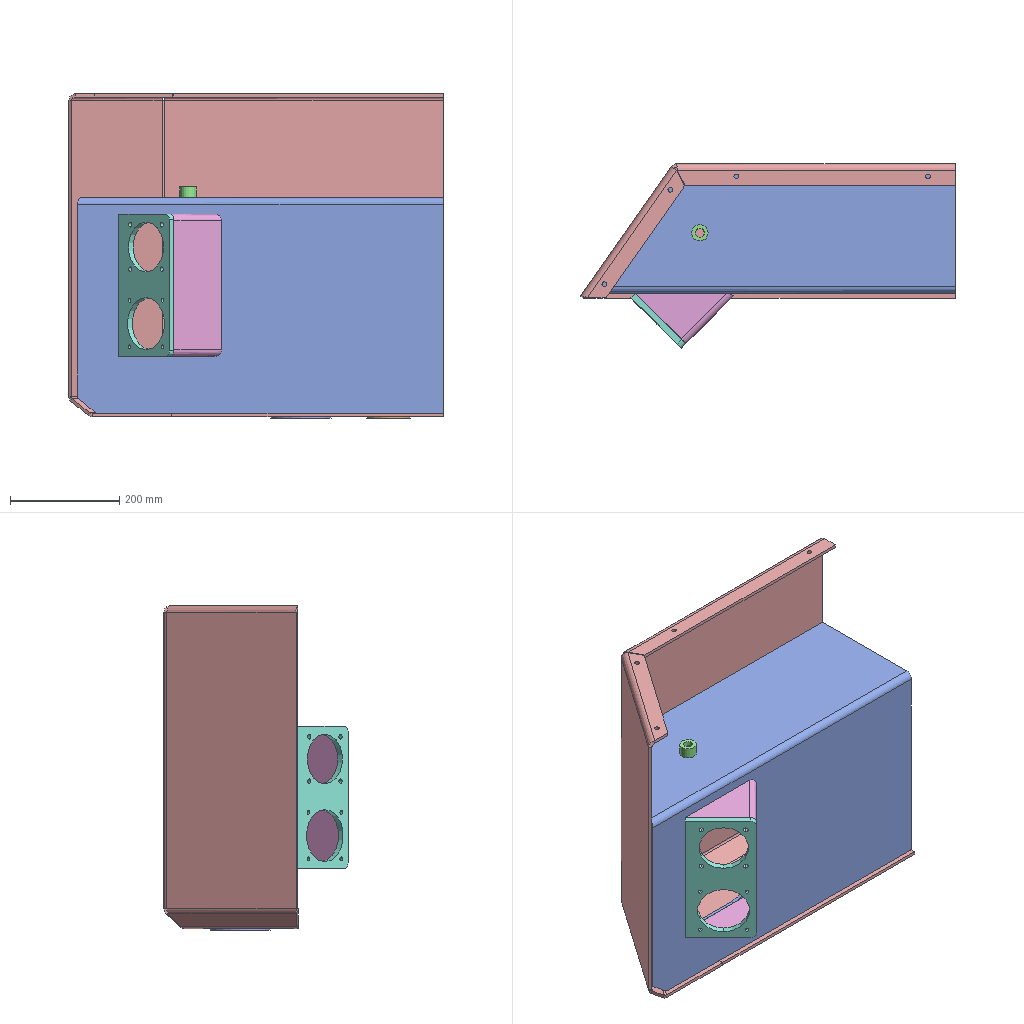Assembly | SolidWorks | 8 different items | 8 placed | box 684 x 336 x 593 mm
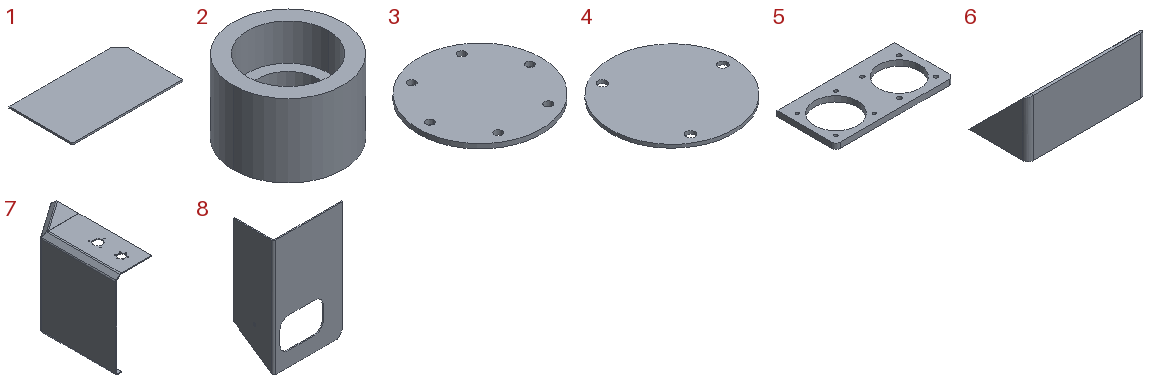Parts list (item | quantity | size | volume | features):
1 | x1 | 388 x 224 x 6 mm | 518873 mm3 | features FlatPattern 1, SMBaseFlange 1, SheetMetal 1
2 | x1 | 30 x 30 x 20 mm | 8198 mm3 | features Extrusion 1, HoleWzd 1, ICE 1
3 | x1 | 80 x 80 x 3 mm | 14726 mm3 | features FlatPattern 1, SMBaseFlange 1, SheetMetal 1
4 | x1 | 110 x 110 x 3 mm | 28058 mm3 | features FlatPattern 1, SMBaseFlange 1, SheetMetal 1
5 | x1 | 260 x 130 x 12 mm | 237513 mm3 | features HoleWzd 2, FlatPattern 1, SMBaseFlange 1, SheetMetal 1
6 | x1 | 260 x 130 x 124 mm | 279794 mm3 | features FlatPattern 1, ICE 1, SMBaseFlange 1, SheetMetal 1
7 | x1 | 244.999 x 684.15 x 590 mm | 3721294 mm3 | features ICE 4, EdgeFlange 3, HoleWzd 2, FlatPattern 1, SMBaseFlange 1, SheetMetal 1
8 | x1 | 394 x 230 x 667.799 mm | 2103650 mm3 | features ICE 3, Chamfer 1, Fillet 1, FlatPattern 1, SMBaseFlange 1, SheetMetal 1
Mates (type | each side: item.copy, entity, surface, feature):
Coincident | 7.1 face plane Base-Flange1 | 8.1 face plane Base-Flange1 | 2 times
Coincident | 7.1 face plane Edge-Flange4 | 8.1 face plane Base-Flange1
Coincident | 8.1 face plane Base-Flange1 | 1.1 face plane Base-Flange1 | 2 times
DistanceDim | 1.1 face plane Base-Flange1 | 7.1 face plane Edge-Flange4
Coincident | 8.1 face plane Base-Flange1 | 6.1 face plane Cut-Extrude1
Coincident | 8.1 face plane Cut-Extrude3 | 6.1 face plane Base-Flange1
Coincident | 8.1 edge | 6.1 edge
Coincident | 6.1 face plane Base-Flange1 | 5.1 face plane Base-Flange1 | 3 times
InPlace | 7.1 face plane Edge-Flange4 | 3.1 plane
InPlace | 7.1 face plane Edge-Flange4 | 4.1 plane
Coincident | 8.1 face plane Base-Flange1 | 2.1 face plane Boss-Extrude1
Concentric | 8.1 face cylinder Cut-Extrude2 | 2.1 face cylinder Boss-Extrude1